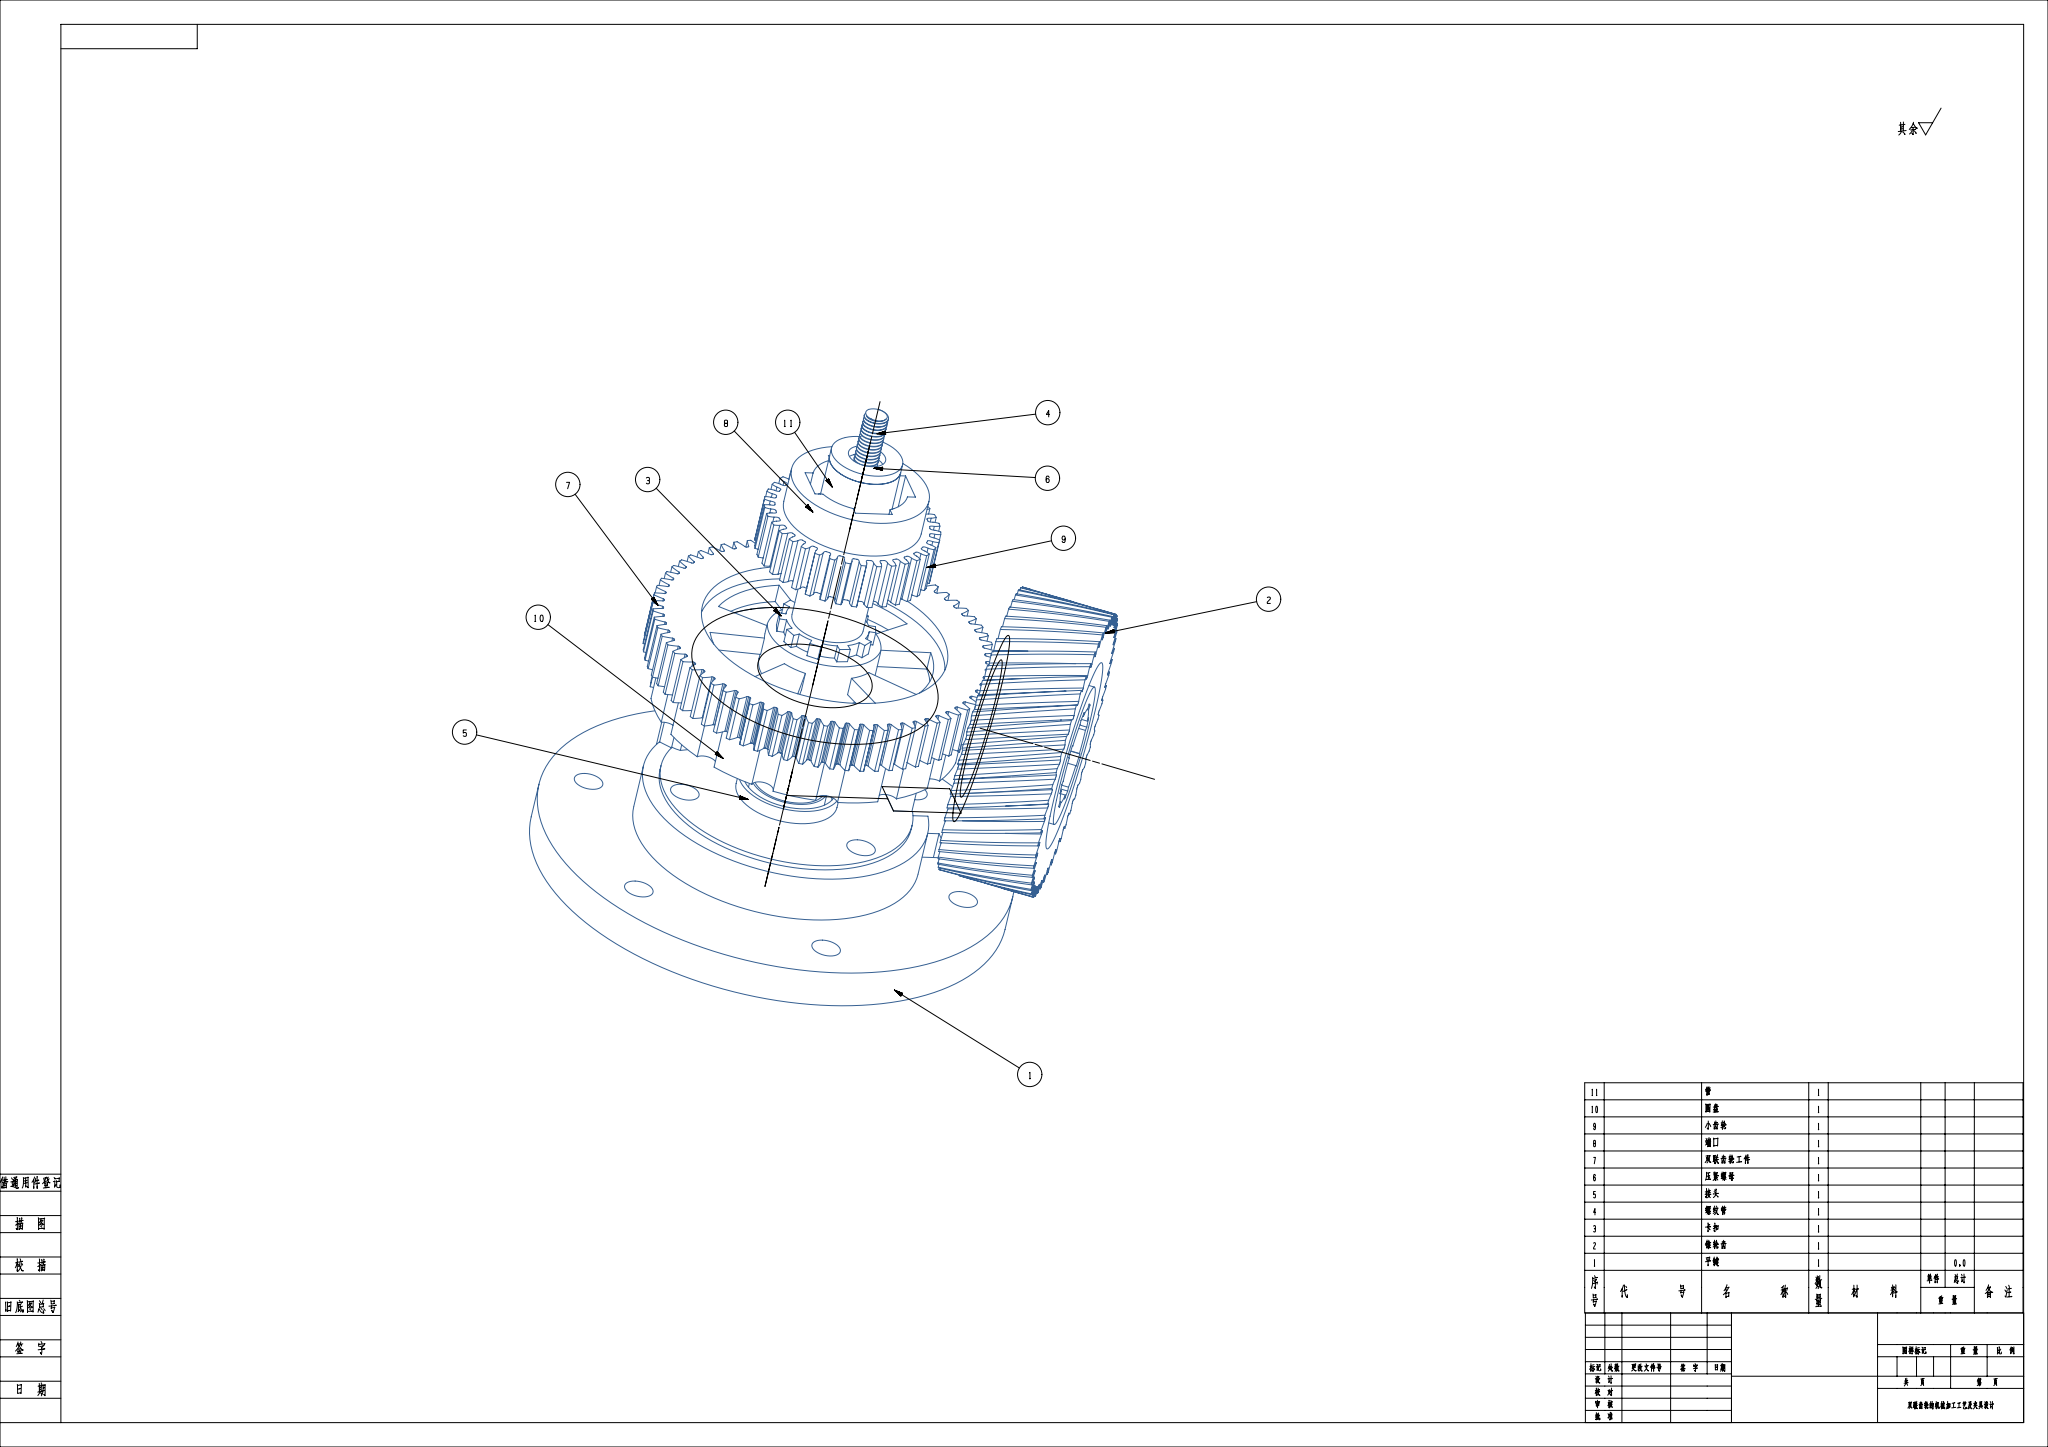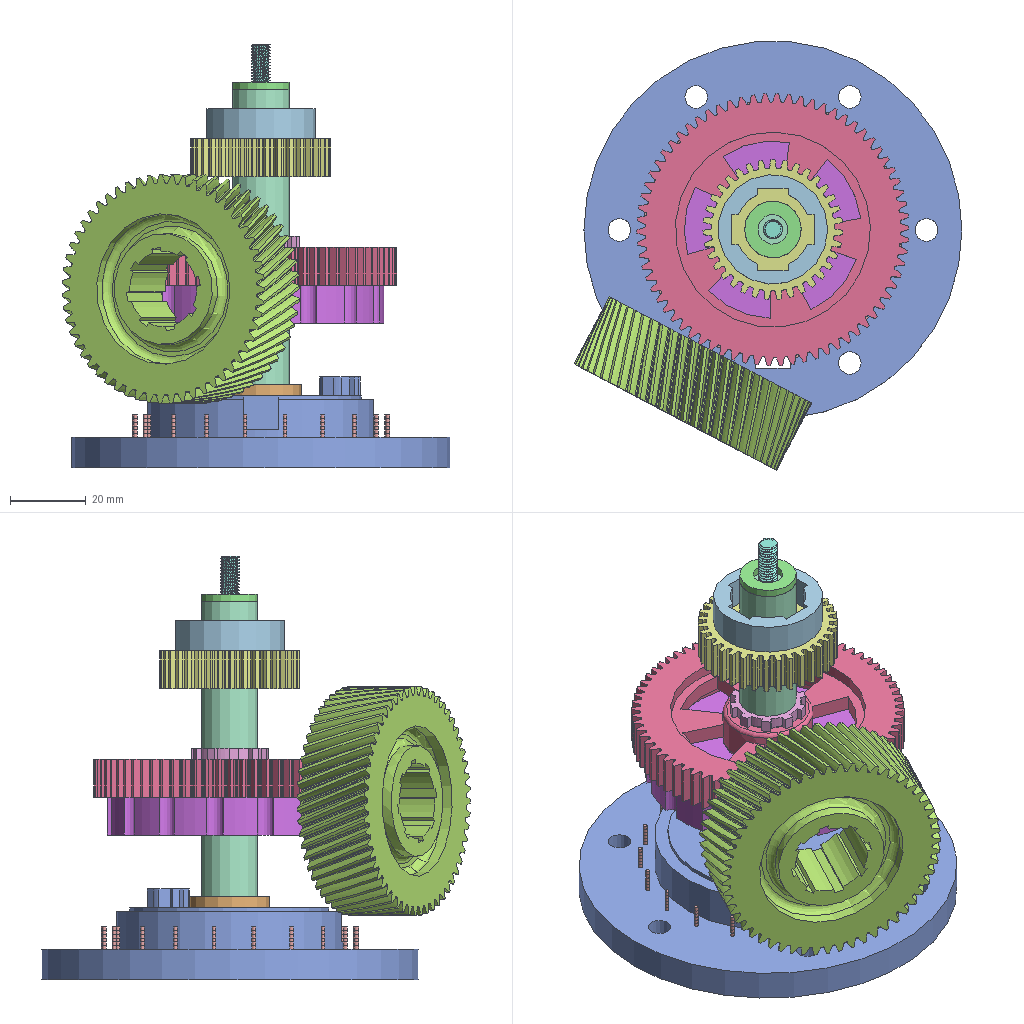Assembly | NX | 13 different items | 132 placed | box 103 x 113 x 112 mm
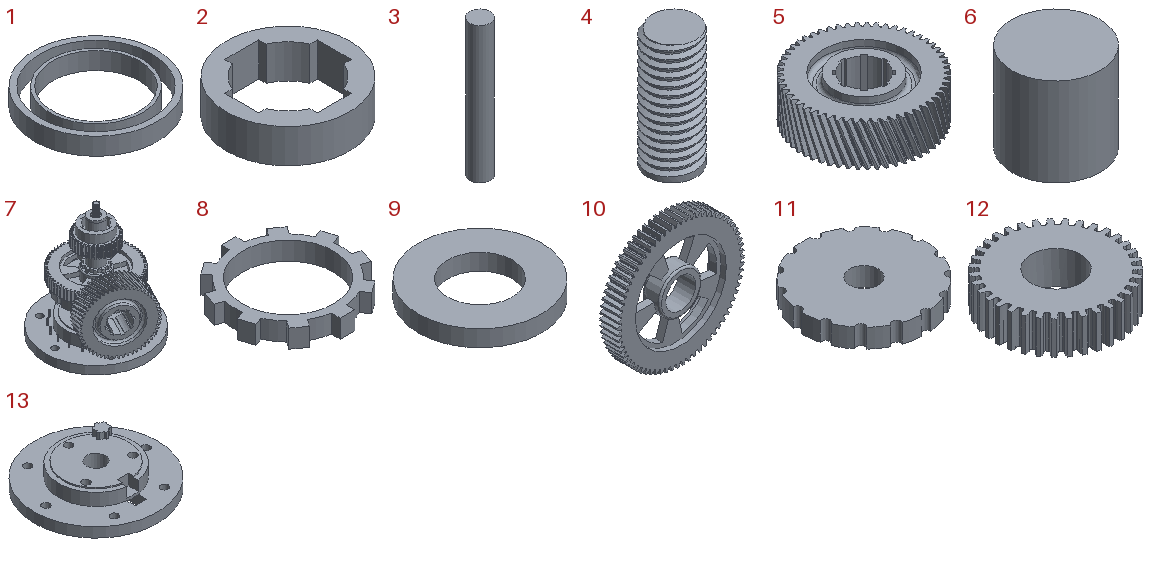Parts list (item | quantity | parent item | size | volume | features):
1 | x1 | in 7 | 21.29 x 21.29 x 3 mm | 261.353 mm3 | features DATUM_CSYS 2, CYLINDER 1, EXTRUDE 1, SKETCH 1
2 | x1 | in 7 | 29 x 29 x 8 mm | 2471 mm3 | features DATUM_CSYS 2, EXTRUDE 1, SKETCH 1
3 | x1 | in 7 | 15 x 15 x 100 mm | 17671 mm3 | features CYLINDER 1, DATUM_CSYS 1
4 | x1 | in 7 | 5 x 5 x 12 mm | 202.074 mm3 | features CYLINDER 1, DATUM_CSYS 1, THREADS 1
5 | x1 | in 7 | - | 41545 mm3 | features BREP 55, META 55, DATUM_CSYS 3, EXTRUDE 3, SKETCH 2, BLEND 1, CYLINDER 1, FSET 1
6 | x120 | in 7 | 1 x 1 x 1 mm | 0.7854 mm3 | features CYLINDER 1, DATUM_CSYS 1
7 | x1 | - | - | 209472 mm3 | features BREP 160, META 160, DATUM_CSYS 26, EXTRUDE 17, SKETCH 14, CYLINDER 11, FSET 3, BLEND 2, REPLACE_FACE 2, OFFSET_REGION 1, THREADS 1
8 | x1 | in 7 | 20.095 x 20.159 x 3 mm | 289.163 mm3 | features DATUM_CSYS 2, EXTRUDE 1, SKETCH 1
9 | x1 | in 7 | 15 x 15 x 2 mm | 256.846 mm3 | features DATUM_CSYS 2, EXTRUDE 1, OFFSET_REGION 1, SKETCH 1
10 | x1 | in 7 | - | 22935 mm3 | features BREP 70, META 70, DATUM_CSYS 4, EXTRUDE 4, SKETCH 3, BLEND 1, CYLINDER 1, FSET 1
11 | x1 | in 7 | 65 x 64.948 x 10 mm | 30179 mm3 | features DATUM_CSYS 2, CYLINDER 1, EXTRUDE 1, SKETCH 1
12 | x1 | in 7 | 37 x 37 x 10 mm | 7712 mm3 | features BREP 35, META 35, DATUM_CSYS 2, CYLINDER 1, EXTRUDE 1, FSET 1, SKETCH 1
13 | x1 | in 7 | 100 x 100 x 24 mm | 85800 mm3 | features DATUM_CSYS 4, EXTRUDE 4, CYLINDER 3, SKETCH 3, REPLACE_FACE 2
Mates (type | each side: item.copy, entity, surface, feature):
Fix | 13.1 component
Concentric | 3.1 | 13.1
AlignLock | 11.1 | 3.1
Concentric | 10.1 | 11.1
Touch | 5.1 | 10.1
Distance | 5.1 | 11.1
Distance | 5.1 | 10.1
Concentric | 8.1 | 10.1
Concentric | 4.1 | 3.1
Concentric | 9.1 | 3.1
Concentric | 1.1 | 13.1
AlignLock | 12.1 | 4.1
Distance | 12.1 | 4.1
Concentric | 2.1 | 12.1
Touch | 6.1 | 13.1
Parallel | 6.1 | 13.1